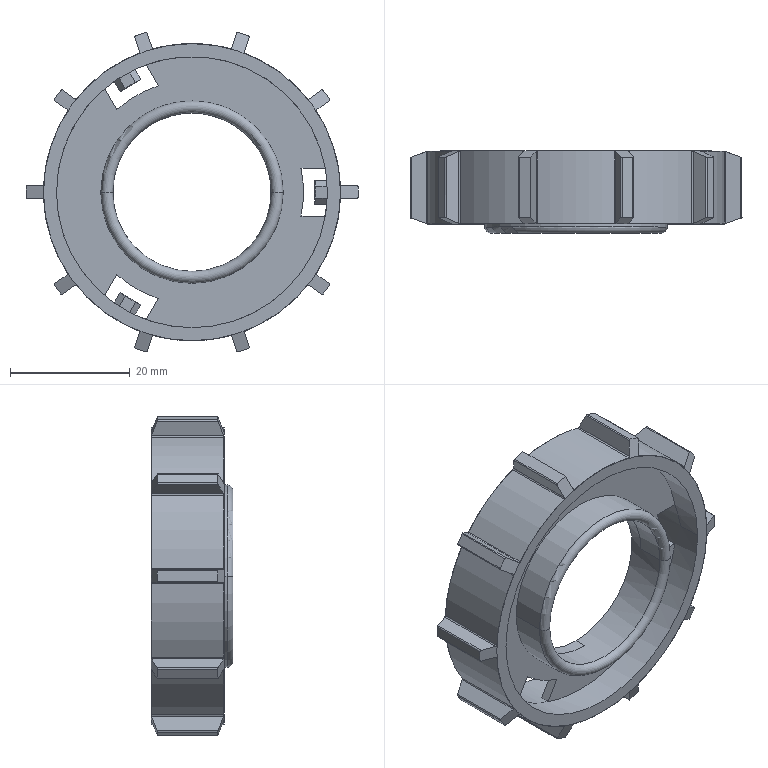Part | STEP file | MSBR-31 | 1 solid | 129 faces | box 55.5 x 13.7 x 53.411 mm | volume 7229 mm3 | cylinder 63 | plane 56 | torus 6 | cone 4 | commonest cylinder face diameters 0.4 x39 49.7 x10 37.3 x3 41.3 x3 26.5 x2 30.5 x2